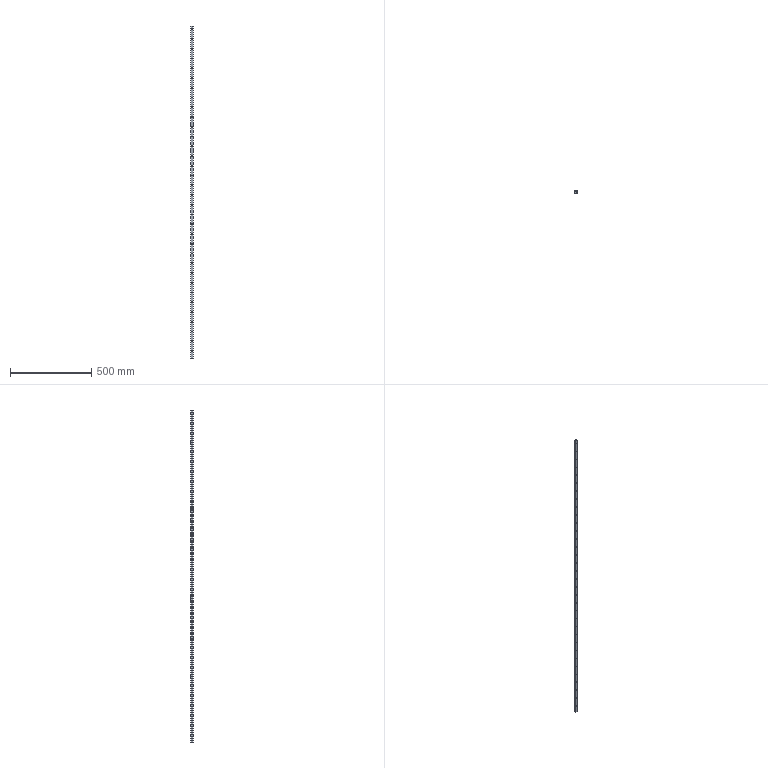Part | SolidWorks | features BaseBody 1, ICE 1 | 1 solid | 196 faces | box 15 x 12.5 x 2043 mm | volume 344620 mm3 | cylinder 142 | plane 54 | commonest cylinder face diameters 4.5 x68 7.5 x68 1.115 x6